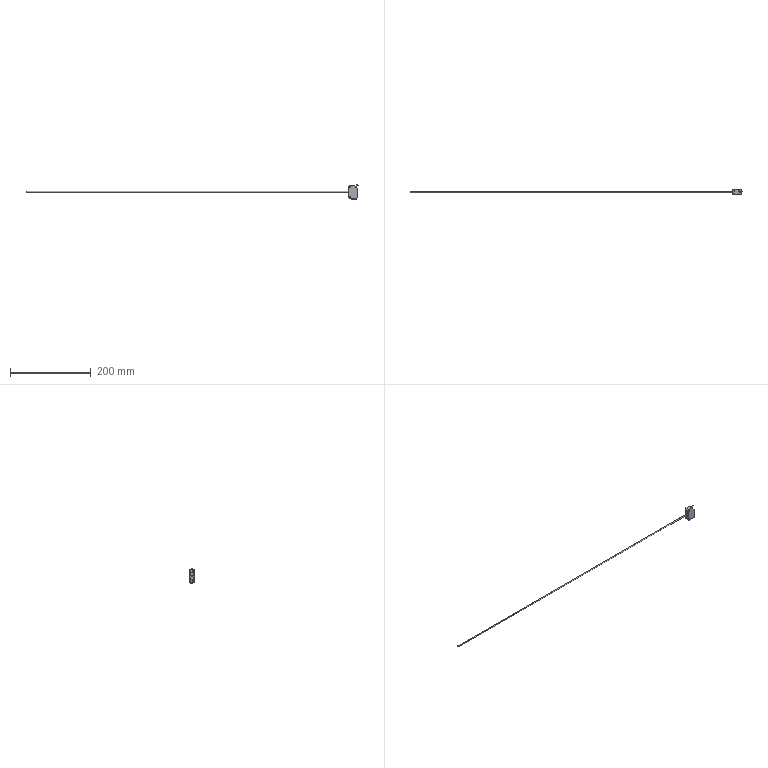Part | SolidWorks | features Boss 4, Chamfer 3, Fillet 3, Cut 2, Dome 2, Extrusion 1, HoleWzd 1, ICE 1 | 2 solids | 67 faces | box 822.394 x 11.2 x 35.904 mm | volume 12330 mm3 | plane 26 | cylinder 25 | cone 8 | torus 4 | sphere 4 | commonest cylinder face diameters 2.5 x4 3.5 x4 3.9 x4 4 x4 3 x2 3.7 x2